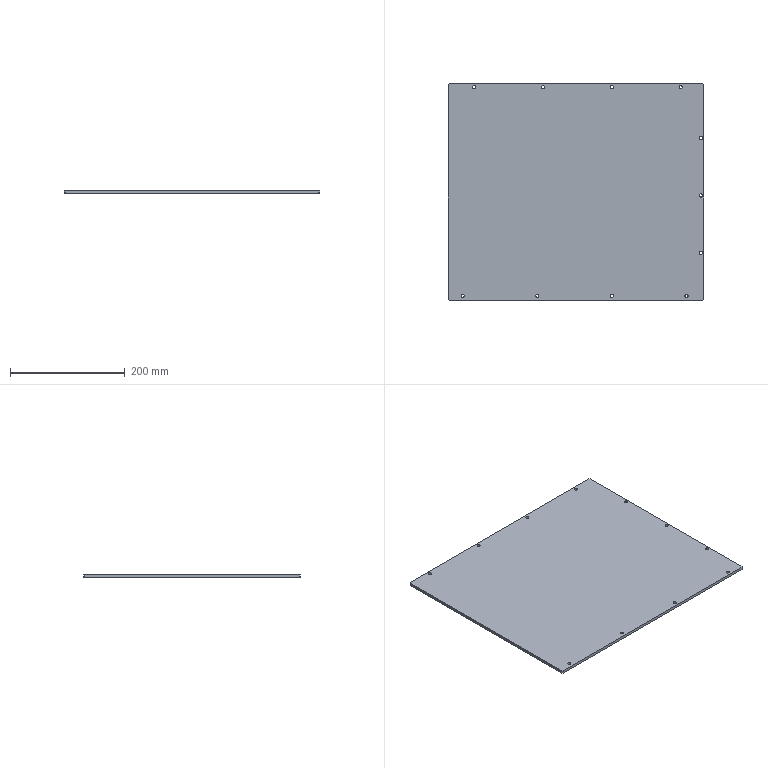Part | SolidWorks | features Extrusion 1, Fillet 1, HoleWzd 1 | 1 solid | 32 faces | box 445 x 377 x 5 mm | volume 837478 mm3 | cylinder 22 | plane 10 | commonest cylinder face diameters 5.5 x22
STEP:
#1=CARTESIAN_POINT('',(-180.25,182.5,0.));
#2=VERTEX_POINT('',#1);
#3=CARTESIAN_POINT('',(-174.75,182.5,0.));
#4=VERTEX_POINT('',#3);
#5=CARTESIAN_POINT('',(-177.5,182.5,0.));
#6=DIRECTION('',(0.,0.,1.));
#7=DIRECTION('',(1.,0.,0.));
#8=AXIS2_PLACEMENT_3D('',#5,#6,#7);
#9=CIRCLE('',#8,2.75);
#10=EDGE_CURVE('',#2,#4,#9,.T.);
#11=ORIENTED_EDGE('',*,*,#10,.F.);
#12=CARTESIAN_POINT('',(-180.25,182.5,5.));
#13=VERTEX_POINT('',#12);
#14=CARTESIAN_POINT('',(-180.25,182.5,5.));
#15=DIRECTION('',(0.,0.,1.));
#16=VECTOR('',#15,1000.);
#17=LINE('',#14,#16);
#18=EDGE_CURVE('',#2,#13,#17,.T.);
#19=ORIENTED_EDGE('',*,*,#18,.T.);
#20=CARTESIAN_POINT('',(-174.75,182.5,5.));
#21=VERTEX_POINT('',#20);
#22=CARTESIAN_POINT('',(-177.5,182.5,5.));
#23=DIRECTION('',(0.,0.,1.));
#24=DIRECTION('',(1.,0.,0.));
#25=AXIS2_PLACEMENT_3D('',#22,#23,#24);
#26=CIRCLE('',#25,2.75);
#27=EDGE_CURVE('',#13,#21,#26,.T.);
#28=ORIENTED_EDGE('',*,*,#27,.T.);
#29=CARTESIAN_POINT('',(-174.75,182.5,5.));
#30=DIRECTION('',(0.,0.,1.));
#31=VECTOR('',#30,1000.);
#32=LINE('',#29,#31);
#33=EDGE_CURVE('',#4,#21,#32,.T.);
#34=ORIENTED_EDGE('',*,*,#33,.F.);
#35=EDGE_LOOP('',(#11,#19,#28,#34));
#36=FACE_OUTER_BOUND('',#35,.T.);
#37=CARTESIAN_POINT('',(-177.5,182.5,5.));
#38=DIRECTION('',(0.,0.,1.));
#39=DIRECTION('',(1.,0.,0.));
#40=AXIS2_PLACEMENT_3D('',#37,#38,#39);
#41=CYLINDRICAL_SURFACE('',#40,2.75);
#42=ADVANCED_FACE('',(#36),#41,.F.);
#43=CARTESIAN_POINT('',(-60.25,182.5,0.));
#44=VERTEX_POINT('',#43);
#45=CARTESIAN_POINT('',(-54.75,182.5,0.));
#46=VERTEX_POINT('',#45);
#47=CARTESIAN_POINT('',(-57.5,182.5,0.));
#48=DIRECTION('',(0.,0.,1.));
#49=DIRECTION('',(1.,0.,0.));
#50=AXIS2_PLACEMENT_3D('',#47,#48,#49);
#51=CIRCLE('',#50,2.75);
#52=EDGE_CURVE('',#44,#46,#51,.T.);
#53=ORIENTED_EDGE('',*,*,#52,.F.);
#54=CARTESIAN_POINT('',(-60.25,182.5,5.));
#55=VERTEX_POINT('',#54);
#56=CARTESIAN_POINT('',(-60.25,182.5,5.));
#57=DIRECTION('',(0.,0.,1.));
#58=VECTOR('',#57,1000.);
#59=LINE('',#56,#58);
#60=EDGE_CURVE('',#44,#55,#59,.T.);
#61=ORIENTED_EDGE('',*,*,#60,.T.);
#62=CARTESIAN_POINT('',(-54.75,182.5,5.));
#63=VERTEX_POINT('',#62);
#64=CARTESIAN_POINT('',(-57.5,182.5,5.));
#65=DIRECTION('',(0.,0.,1.));
#66=DIRECTION('',(1.,0.,0.));
#67=AXIS2_PLACEMENT_3D('',#64,#65,#66);
#68=CIRCLE('',#67,2.75);
#69=EDGE_CURVE('',#55,#63,#68,.T.);
#70=ORIENTED_EDGE('',*,*,#69,.T.);
#71=CARTESIAN_POINT('',(-54.75,182.5,5.));
#72=DIRECTION('',(0.,0.,1.));
#73=VECTOR('',#72,1000.);
#74=LINE('',#71,#73);
#75=EDGE_CURVE('',#46,#63,#74,.T.);
#76=ORIENTED_EDGE('',*,*,#75,.F.);
#77=EDGE_LOOP('',(#53,#61,#70,#76));
#78=FACE_OUTER_BOUND('',#77,.T.);
#79=CARTESIAN_POINT('',(-57.5,182.5,5.));
#80=DIRECTION('',(0.,0.,1.));
#81=DIRECTION('',(1.,0.,0.));
#82=AXIS2_PLACEMENT_3D('',#79,#80,#81);
#83=CYLINDRICAL_SURFACE('',#82,2.75);
#84=ADVANCED_FACE('',(#78),#83,.F.);
#85=CARTESIAN_POINT('',(59.75,182.5,0.));
#86=VERTEX_POINT('',#85);
#87=CARTESIAN_POINT('',(65.25,182.5,0.));
#88=VERTEX_POINT('',#87);
#89=CARTESIAN_POINT('',(62.5,182.5,0.));
#90=DIRECTION('',(0.,0.,1.));
#91=DIRECTION('',(1.,0.,0.));
#92=AXIS2_PLACEMENT_3D('',#89,#90,#91);
#93=CIRCLE('',#92,2.75);
#94=EDGE_CURVE('',#86,#88,#93,.T.);
#95=ORIENTED_EDGE('',*,*,#94,.F.);
#96=CARTESIAN_POINT('',(59.75,182.5,5.));
#97=VERTEX_POINT('',#96);
#98=CARTESIAN_POINT('',(59.75,182.5,5.));
#99=DIRECTION('',(0.,0.,1.));
#100=VECTOR('',#99,1000.);
#101=LINE('',#98,#100);
#102=EDGE_CURVE('',#86,#97,#101,.T.);
#103=ORIENTED_EDGE('',*,*,#102,.T.);
#104=CARTESIAN_POINT('',(65.25,182.5,5.));
#105=VERTEX_POINT('',#104);
#106=CARTESIAN_POINT('',(62.5,182.5,5.));
#107=DIRECTION('',(0.,0.,1.));
#108=DIRECTION('',(1.,0.,0.));
#109=AXIS2_PLACEMENT_3D('',#106,#107,#108);
#110=CIRCLE('',#109,2.75);
#111=EDGE_CURVE('',#97,#105,#110,.T.);
#112=ORIENTED_EDGE('',*,*,#111,.T.);
#113=CARTESIAN_POINT('',(65.25,182.5,5.));
#114=DIRECTION('',(0.,0.,1.));
#115=VECTOR('',#114,1000.);
#116=LINE('',#113,#115);
#117=EDGE_CURVE('',#88,#105,#116,.T.);
#118=ORIENTED_EDGE('',*,*,#117,.F.);
#119=EDGE_LOOP('',(#95,#103,#112,#118));
#120=FACE_OUTER_BOUND('',#119,.T.);
#121=CARTESIAN_POINT('',(62.5,182.5,5.));
#122=DIRECTION('',(0.,0.,1.));
#123=DIRECTION('',(1.,0.,0.));
#124=AXIS2_PLACEMENT_3D('',#121,#122,#123);
#125=CYLINDRICAL_SURFACE('',#124,2.75);
#126=ADVANCED_FACE('',(#120),#125,.F.);
#127=CARTESIAN_POINT('',(179.75,182.5,0.));
#128=VERTEX_POINT('',#127);
#129=CARTESIAN_POINT('',(185.25,182.5,0.));
#130=VERTEX_POINT('',#129);
#131=CARTESIAN_POINT('',(182.5,182.5,0.));
#132=DIRECTION('',(0.,0.,1.));
#133=DIRECTION('',(1.,0.,0.));
#134=AXIS2_PLACEMENT_3D('',#131,#132,#133);
#135=CIRCLE('',#134,2.75);
#136=EDGE_CURVE('',#128,#130,#135,.T.);
#137=ORIENTED_EDGE('',*,*,#136,.F.);
#138=CARTESIAN_POINT('',(179.75,182.5,5.));
#139=VERTEX_POINT('',#138);
#140=CARTESIAN_POINT('',(179.75,182.5,5.));
#141=DIRECTION('',(0.,0.,1.));
#142=VECTOR('',#141,1000.);
#143=LINE('',#140,#142);
#144=EDGE_CURVE('',#128,#139,#143,.T.);
#145=ORIENTED_EDGE('',*,*,#144,.T.);
#146=CARTESIAN_POINT('',(185.25,182.5,5.));
#147=VERTEX_POINT('',#146);
#148=CARTESIAN_POINT('',(182.5,182.5,5.));
#149=DIRECTION('',(0.,0.,1.));
#150=DIRECTION('',(1.,0.,0.));
#151=AXIS2_PLACEMENT_3D('',#148,#149,#150);
#152=CIRCLE('',#151,2.75);
#153=EDGE_CURVE('',#139,#147,#152,.T.);
#154=ORIENTED_EDGE('',*,*,#153,.T.);
#155=CARTESIAN_POINT('',(185.25,182.5,5.));
#156=DIRECTION('',(0.,0.,1.));
#157=VECTOR('',#156,1000.);
#158=LINE('',#155,#157);
#159=EDGE_CURVE('',#130,#147,#158,.T.);
#160=ORIENTED_EDGE('',*,*,#159,.F.);
#161=EDGE_LOOP('',(#137,#145,#154,#160));
#162=FACE_OUTER_BOUND('',#161,.T.);
#163=CARTESIAN_POINT('',(182.5,182.5,5.));
#164=DIRECTION('',(0.,0.,1.));
#165=DIRECTION('',(1.,0.,0.));
#166=AXIS2_PLACEMENT_3D('',#163,#164,#165);
#167=CYLINDRICAL_SURFACE('',#166,2.75);
#168=ADVANCED_FACE('',(#162),#167,.F.);
#169=CARTESIAN_POINT('',(-200.25,-181.,0.));
#170=VERTEX_POINT('',#169);
#171=CARTESIAN_POINT('',(-194.75,-181.,0.));
#172=VERTEX_POINT('',#171);
#173=CARTESIAN_POINT('',(-197.5,-181.,0.));
#174=DIRECTION('',(0.,0.,1.));
#175=DIRECTION('',(1.,0.,0.));
#176=AXIS2_PLACEMENT_3D('',#173,#174,#175);
#177=CIRCLE('',#176,2.75);
#178=EDGE_CURVE('',#170,#172,#177,.T.);
#179=ORIENTED_EDGE('',*,*,#178,.F.);
#180=CARTESIAN_POINT('',(-200.25,-181.,5.));
#181=VERTEX_POINT('',#180);
#182=CARTESIAN_POINT('',(-200.25,-181.,5.));
#183=DIRECTION('',(0.,0.,1.));
#184=VECTOR('',#183,1000.);
#185=LINE('',#182,#184);
#186=EDGE_CURVE('',#170,#181,#185,.T.);
#187=ORIENTED_EDGE('',*,*,#186,.T.);
#188=CARTESIAN_POINT('',(-194.75,-181.,5.));
#189=VERTEX_POINT('',#188);
#190=CARTESIAN_POINT('',(-197.5,-181.,5.));
#191=DIRECTION('',(0.,0.,1.));
#192=DIRECTION('',(1.,0.,0.));
#193=AXIS2_PLACEMENT_3D('',#190,#191,#192);
#194=CIRCLE('',#193,2.75);
#195=EDGE_CURVE('',#181,#189,#194,.T.);
#196=ORIENTED_EDGE('',*,*,#195,.T.);
#197=CARTESIAN_POINT('',(-194.75,-181.,5.));
#198=DIRECTION('',(0.,0.,1.));
#199=VECTOR('',#198,1000.);
#200=LINE('',#197,#199);
#201=EDGE_CURVE('',#172,#189,#200,.T.);
#202=ORIENTED_EDGE('',*,*,#201,.F.);
#203=EDGE_LOOP('',(#179,#187,#196,#202));
#204=FACE_OUTER_BOUND('',#203,.T.);
#205=CARTESIAN_POINT('',(-197.5,-181.,5.));
#206=DIRECTION('',(0.,0.,1.));
#207=DIRECTION('',(1.,0.,0.));
#208=AXIS2_PLACEMENT_3D('',#205,#206,#207);
#209=CYLINDRICAL_SURFACE('',#208,2.75);
#210=ADVANCED_FACE('',(#204),#209,.F.);
#211=CARTESIAN_POINT('',(-70.25,-181.,0.));
#212=VERTEX_POINT('',#211);
#213=CARTESIAN_POINT('',(-64.75,-181.,0.));
#214=VERTEX_POINT('',#213);
#215=CARTESIAN_POINT('',(-67.5,-181.,0.));
#216=DIRECTION('',(0.,0.,1.));
#217=DIRECTION('',(1.,0.,0.));
#218=AXIS2_PLACEMENT_3D('',#215,#216,#217);
#219=CIRCLE('',#218,2.75);
#220=EDGE_CURVE('',#212,#214,#219,.T.);
#221=ORIENTED_EDGE('',*,*,#220,.F.);
#222=CARTESIAN_POINT('',(-70.25,-181.,5.));
#223=VERTEX_POINT('',#222);
#224=CARTESIAN_POINT('',(-70.25,-181.,5.));
#225=DIRECTION('',(0.,0.,1.));
#226=VECTOR('',#225,1000.);
#227=LINE('',#224,#226);
#228=EDGE_CURVE('',#212,#223,#227,.T.);
#229=ORIENTED_EDGE('',*,*,#228,.T.);
#230=CARTESIAN_POINT('',(-64.75,-181.,5.));
#231=VERTEX_POINT('',#230);
#232=CARTESIAN_POINT('',(-67.5,-181.,5.));
#233=DIRECTION('',(0.,0.,1.));
#234=DIRECTION('',(1.,0.,0.));
#235=AXIS2_PLACEMENT_3D('',#232,#233,#234);
#236=CIRCLE('',#235,2.75);
#237=EDGE_CURVE('',#223,#231,#236,.T.);
#238=ORIENTED_EDGE('',*,*,#237,.T.);
#239=CARTESIAN_POINT('',(-64.75,-181.,5.));
#240=DIRECTION('',(0.,0.,1.));
#241=VECTOR('',#240,1000.);
#242=LINE('',#239,#241);
#243=EDGE_CURVE('',#214,#231,#242,.T.);
#244=ORIENTED_EDGE('',*,*,#243,.F.);
#245=EDGE_LOOP('',(#221,#229,#238,#244));
#246=FACE_OUTER_BOUND('',#245,.T.);
#247=CARTESIAN_POINT('',(-67.5,-181.,5.));
#248=DIRECTION('',(0.,0.,1.));
#249=DIRECTION('',(1.,0.,0.));
#250=AXIS2_PLACEMENT_3D('',#247,#248,#249);
#251=CYLINDRICAL_SURFACE('',#250,2.75);
#252=ADVANCED_FACE('',(#246),#251,.F.);
#253=CARTESIAN_POINT('',(59.75,-181.,0.));
#254=VERTEX_POINT('',#253);
#255=CARTESIAN_POINT('',(65.25,-181.,0.));
#256=VERTEX_POINT('',#255);
#257=CARTESIAN_POINT('',(62.5,-181.,0.));
#258=DIRECTION('',(0.,0.,1.));
#259=DIRECTION('',(1.,0.,0.));
#260=AXIS2_PLACEMENT_3D('',#257,#258,#259);
#261=CIRCLE('',#260,2.75);
#262=EDGE_CURVE('',#254,#256,#261,.T.);
#263=ORIENTED_EDGE('',*,*,#262,.F.);
#264=CARTESIAN_POINT('',(59.75,-181.,5.));
#265=VERTEX_POINT('',#264);
#266=CARTESIAN_POINT('',(59.75,-181.,5.));
#267=DIRECTION('',(0.,0.,1.));
#268=VECTOR('',#267,1000.);
#269=LINE('',#266,#268);
#270=EDGE_CURVE('',#254,#265,#269,.T.);
#271=ORIENTED_EDGE('',*,*,#270,.T.);
#272=CARTESIAN_POINT('',(65.25,-181.,5.));
#273=VERTEX_POINT('',#272);
#274=CARTESIAN_POINT('',(62.5,-181.,5.));
#275=DIRECTION('',(0.,0.,1.));
#276=DIRECTION('',(1.,0.,0.));
#277=AXIS2_PLACEMENT_3D('',#274,#275,#276);
#278=CIRCLE('',#277,2.75);
#279=EDGE_CURVE('',#265,#273,#278,.T.);
#280=ORIENTED_EDGE('',*,*,#279,.T.);
#281=CARTESIAN_POINT('',(65.25,-181.,5.));
#282=DIRECTION('',(0.,0.,1.));
#283=VECTOR('',#282,1000.);
#284=LINE('',#281,#283);
#285=EDGE_CURVE('',#256,#273,#284,.T.);
#286=ORIENTED_EDGE('',*,*,#285,.F.);
#287=EDGE_LOOP('',(#263,#271,#280,#286));
#288=FACE_OUTER_BOUND('',#287,.T.);
#289=CARTESIAN_POINT('',(62.5,-181.,5.));
#290=DIRECTION('',(0.,0.,1.));
#291=DIRECTION('',(1.,0.,0.));
#292=AXIS2_PLACEMENT_3D('',#289,#290,#291);
#293=CYLINDRICAL_SURFACE('',#292,2.75);
#294=ADVANCED_FACE('',(#288),#293,.F.);
#295=CARTESIAN_POINT('',(189.75,-181.,0.));
#296=VERTEX_POINT('',#295);
#297=CARTESIAN_POINT('',(195.25,-181.,0.));
#298=VERTEX_POINT('',#297);
#299=CARTESIAN_POINT('',(192.5,-181.,0.));
#300=DIRECTION('',(0.,0.,1.));
#301=DIRECTION('',(1.,0.,0.));
#302=AXIS2_PLACEMENT_3D('',#299,#300,#301);
#303=CIRCLE('',#302,2.75);
#304=EDGE_CURVE('',#296,#298,#303,.T.);
#305=ORIENTED_EDGE('',*,*,#304,.F.);
#306=CARTESIAN_POINT('',(189.75,-181.,5.));
#307=VERTEX_POINT('',#306);
#308=CARTESIAN_POINT('',(189.75,-181.,5.));
#309=DIRECTION('',(0.,0.,1.));
#310=VECTOR('',#309,1000.);
#311=LINE('',#308,#310);
#312=EDGE_CURVE('',#296,#307,#311,.T.);
#313=ORIENTED_EDGE('',*,*,#312,.T.);
#314=CARTESIAN_POINT('',(195.25,-181.,5.));
#315=VERTEX_POINT('',#314);
#316=CARTESIAN_POINT('',(192.5,-181.,5.));
#317=DIRECTION('',(0.,0.,1.));
#318=DIRECTION('',(1.,0.,0.));
#319=AXIS2_PLACEMENT_3D('',#316,#317,#318);
#320=CIRCLE('',#319,2.75);
#321=EDGE_CURVE('',#307,#315,#320,.T.);
#322=ORIENTED_EDGE('',*,*,#321,.T.);
#323=CARTESIAN_POINT('',(195.25,-181.,5.));
#324=DIRECTION('',(0.,0.,1.));
#325=VECTOR('',#324,1000.);
#326=LINE('',#323,#325);
#327=EDGE_CURVE('',#298,#315,#326,.T.);
#328=ORIENTED_EDGE('',*,*,#327,.F.);
#329=EDGE_LOOP('',(#305,#313,#322,#328));
#330=FACE_OUTER_BOUND('',#329,.T.);
#331=CARTESIAN_POINT('',(192.5,-181.,5.));
#332=DIRECTION('',(0.,0.,1.));
#333=DIRECTION('',(1.,0.,0.));
#334=AXIS2_PLACEMENT_3D('',#331,#332,#333);
#335=CYLINDRICAL_SURFACE('',#334,2.75);
#336=ADVANCED_FACE('',(#330),#335,.F.);
#337=CARTESIAN_POINT('',(214.75,-106.,0.));
#338=VERTEX_POINT('',#337);
#339=CARTESIAN_POINT('',(220.25,-106.,0.));
#340=VERTEX_POINT('',#339);
#341=CARTESIAN_POINT('',(217.5,-106.,0.));
#342=DIRECTION('',(0.,0.,1.));
#343=DIRECTION('',(1.,0.,0.));
#344=AXIS2_PLACEMENT_3D('',#341,#342,#343);
#345=CIRCLE('',#344,2.75);
#346=EDGE_CURVE('',#338,#340,#345,.T.);
#347=ORIENTED_EDGE('',*,*,#346,.F.);
#348=CARTESIAN_POINT('',(214.75,-106.,5.));
#349=VERTEX_POINT('',#348);
#350=CARTESIAN_POINT('',(214.75,-106.,5.));
#351=DIRECTION('',(0.,0.,1.));
#352=VECTOR('',#351,1000.);
#353=LINE('',#350,#352);
#354=EDGE_CURVE('',#338,#349,#353,.T.);
#355=ORIENTED_EDGE('',*,*,#354,.T.);
#356=CARTESIAN_POINT('',(220.25,-106.,5.));
#357=VERTEX_POINT('',#356);
#358=CARTESIAN_POINT('',(217.5,-106.,5.));
#359=DIRECTION('',(0.,0.,1.));
#360=DIRECTION('',(1.,0.,0.));
#361=AXIS2_PLACEMENT_3D('',#358,#359,#360);
#362=CIRCLE('',#361,2.75);
#363=EDGE_CURVE('',#349,#357,#362,.T.);
#364=ORIENTED_EDGE('',*,*,#363,.T.);
#365=CARTESIAN_POINT('',(220.25,-106.,5.));
#366=DIRECTION('',(0.,0.,1.));
#367=VECTOR('',#366,1000.);
#368=LINE('',#365,#367);
#369=EDGE_CURVE('',#340,#357,#368,.T.);
#370=ORIENTED_EDGE('',*,*,#369,.F.);
#371=EDGE_LOOP('',(#347,#355,#364,#370));
#372=FACE_OUTER_BOUND('',#371,.T.);
#373=CARTESIAN_POINT('',(217.5,-106.,5.));
#374=DIRECTION('',(0.,0.,1.));
#375=DIRECTION('',(1.,0.,0.));
#376=AXIS2_PLACEMENT_3D('',#373,#374,#375);
#377=CYLINDRICAL_SURFACE('',#376,2.75);
#378=ADVANCED_FACE('',(#372),#377,.F.);
#379=CARTESIAN_POINT('',(214.75,-6.,0.));
#380=VERTEX_POINT('',#379);
#381=CARTESIAN_POINT('',(220.25,-6.,0.));
#382=VERTEX_POINT('',#381);
#383=CARTESIAN_POINT('',(217.5,-6.,0.));
#384=DIRECTION('',(0.,0.,1.));
#385=DIRECTION('',(1.,0.,0.));
#386=AXIS2_PLACEMENT_3D('',#383,#384,#385);
#387=CIRCLE('',#386,2.75);
#388=EDGE_CURVE('',#380,#382,#387,.T.);
#389=ORIENTED_EDGE('',*,*,#388,.F.);
#390=CARTESIAN_POINT('',(214.75,-6.,5.));
#391=VERTEX_POINT('',#390);
#392=CARTESIAN_POINT('',(214.75,-6.,5.));
#393=DIRECTION('',(0.,0.,1.));
#394=VECTOR('',#393,1000.);
#395=LINE('',#392,#394);
#396=EDGE_CURVE('',#380,#391,#395,.T.);
#397=ORIENTED_EDGE('',*,*,#396,.T.);
#398=CARTESIAN_POINT('',(220.25,-6.,5.));
#399=VERTEX_POINT('',#398);
#400=CARTESIAN_POINT('',(217.5,-6.,5.));
#401=DIRECTION('',(0.,0.,1.));
#402=DIRECTION('',(1.,0.,0.));
#403=AXIS2_PLACEMENT_3D('',#400,#401,#402);
#404=CIRCLE('',#403,2.75);
#405=EDGE_CURVE('',#391,#399,#404,.T.);
#406=ORIENTED_EDGE('',*,*,#405,.T.);
#407=CARTESIAN_POINT('',(220.25,-6.,5.));
#408=DIRECTION('',(0.,0.,1.));
#409=VECTOR('',#408,1000.);
#410=LINE('',#407,#409);
#411=EDGE_CURVE('',#382,#399,#410,.T.);
#412=ORIENTED_EDGE('',*,*,#411,.F.);
#413=EDGE_LOOP('',(#389,#397,#406,#412));
#414=FACE_OUTER_BOUND('',#413,.T.);
#415=CARTESIAN_POINT('',(217.5,-6.,5.));
#416=DIRECTION('',(0.,0.,1.));
#417=DIRECTION('',(1.,0.,0.));
#418=AXIS2_PLACEMENT_3D('',#415,#416,#417);
#419=CYLINDRICAL_SURFACE('',#418,2.75);
#420=ADVANCED_FACE('',(#414),#419,.F.);
#421=CARTESIAN_POINT('',(214.75,94.,0.));
#422=VERTEX_POINT('',#421);
#423=CARTESIAN_POINT('',(220.25,94.,0.));
#424=VERTEX_POINT('',#423);
#425=CARTESIAN_POINT('',(217.5,94.,0.));
#426=DIRECTION('',(0.,0.,1.));
#427=DIRECTION('',(1.,0.,0.));
#428=AXIS2_PLACEMENT_3D('',#425,#426,#427);
#429=CIRCLE('',#428,2.75);
#430=EDGE_CURVE('',#422,#424,#429,.T.);
#431=ORIENTED_EDGE('',*,*,#430,.F.);
#432=CARTESIAN_POINT('',(214.75,94.,5.));
#433=VERTEX_POINT('',#432);
#434=CARTESIAN_POINT('',(214.75,94.,5.));
#435=DIRECTION('',(0.,0.,1.));
#436=VECTOR('',#435,1000.);
#437=LINE('',#434,#436);
#438=EDGE_CURVE('',#422,#433,#437,.T.);
#439=ORIENTED_EDGE('',*,*,#438,.T.);
#440=CARTESIAN_POINT('',(220.25,94.,5.));
#441=VERTEX_POINT('',#440);
#442=CARTESIAN_POINT('',(217.5,94.,5.));
#443=DIRECTION('',(0.,0.,1.));
#444=DIRECTION('',(1.,0.,0.));
#445=AXIS2_PLACEMENT_3D('',#442,#443,#444);
#446=CIRCLE('',#445,2.75);
#447=EDGE_CURVE('',#433,#441,#446,.T.);
#448=ORIENTED_EDGE('',*,*,#447,.T.);
#449=CARTESIAN_POINT('',(220.25,94.,5.));
#450=DIRECTION('',(0.,0.,1.));
#451=VECTOR('',#450,1000.);
#452=LINE('',#449,#451);
#453=EDGE_CURVE('',#424,#441,#452,.T.);
#454=ORIENTED_EDGE('',*,*,#453,.F.);
#455=EDGE_LOOP('',(#431,#439,#448,#454));
#456=FACE_OUTER_BOUND('',#455,.T.);
#457=CARTESIAN_POINT('',(217.5,94.,5.));
#458=DIRECTION('',(0.,0.,1.));
#459=DIRECTION('',(1.,0.,0.));
#460=AXIS2_PLACEMENT_3D('',#457,#458,#459);
#461=CYLINDRICAL_SURFACE('',#460,2.75);
#462=ADVANCED_FACE('',(#456),#461,.F.);
#463=CARTESIAN_POINT('',(222.5,-186.5,5.));
#464=VERTEX_POINT('',#463);
#465=CARTESIAN_POINT('',(222.5,186.5,5.));
#466=VERTEX_POINT('',#465);
#467=CARTESIAN_POINT('',(222.5,188.5,5.));
#468=DIRECTION('',(0.,1.,0.));
#469=VECTOR('',#468,1000.);
#470=LINE('',#467,#469);
#471=EDGE_CURVE('',#464,#466,#470,.T.);
#472=ORIENTED_EDGE('',*,*,#471,.F.);
#473=CARTESIAN_POINT('',(222.5,-186.5,0.));
#474=VERTEX_POINT('',#473);
#475=CARTESIAN_POINT('',(222.5,-186.5,5.));
#476=DIRECTION('',(0.,0.,-1.));
#477=VECTOR('',#476,1000.);
#478=LINE('',#475,#477);
#479=EDGE_CURVE('',#464,#474,#478,.T.);
#480=ORIENTED_EDGE('',*,*,#479,.T.);
#481=CARTESIAN_POINT('',(222.5,186.5,0.));
#482=VERTEX_POINT('',#481);
#483=CARTESIAN_POINT('',(222.5,188.5,0.));
#484=DIRECTION('',(0.,1.,0.));
#485=VECTOR('',#484,1000.);
#486=LINE('',#483,#485);
#487=EDGE_CURVE('',#474,#482,#486,.T.);
#488=ORIENTED_EDGE('',*,*,#487,.T.);
#489=CARTESIAN_POINT('',(222.5,186.5,5.));
#490=DIRECTION('',(0.,0.,1.));
#491=VECTOR('',#490,1000.);
#492=LINE('',#489,#491);
#493=EDGE_CURVE('',#482,#466,#492,.T.);
#494=ORIENTED_EDGE('',*,*,#493,.T.);
#495=EDGE_LOOP('',(#472,#480,#488,#494));
#496=FACE_OUTER_BOUND('',#495,.T.);
#497=CARTESIAN_POINT('',(222.5,188.5,5.));
#498=DIRECTION('',(-1.,0.,0.));
#499=DIRECTION('',(0.,-1.,0.));
#500=AXIS2_PLACEMENT_3D('',#497,#498,#499);
#501=PLANE('',#500);
#502=ADVANCED_FACE('',(#496),#501,.F.);
#503=CARTESIAN_POINT('',(220.5,188.5,0.));
#504=VERTEX_POINT('',#503);
#505=CARTESIAN_POINT('',(-220.5,188.5,0.));
#506=VERTEX_POINT('',#505);
#507=CARTESIAN_POINT('',(-222.5,188.5,0.));
#508=DIRECTION('',(-1.,0.,0.));
#509=VECTOR('',#508,1000.);
#510=LINE('',#507,#509);
#511=EDGE_CURVE('',#504,#506,#510,.T.);
#512=ORIENTED_EDGE('',*,*,#511,.T.);
#513=CARTESIAN_POINT('',(-220.5,188.5,5.));
#514=VERTEX_POINT('',#513);
#515=CARTESIAN_POINT('',(-220.5,188.5,5.));
#516=DIRECTION('',(0.,0.,1.));
#517=VECTOR('',#516,1000.);
#518=LINE('',#515,#517);
#519=EDGE_CURVE('',#506,#514,#518,.T.);
#520=ORIENTED_EDGE('',*,*,#519,.T.);
#521=CARTESIAN_POINT('',(220.5,188.5,5.));
#522=VERTEX_POINT('',#521);
#523=CARTESIAN_POINT('',(-222.5,188.5,5.));
#524=DIRECTION('',(-1.,0.,0.));
#525=VECTOR('',#524,1000.);
#526=LINE('',#523,#525);
#527=EDGE_CURVE('',#522,#514,#526,.T.);
#528=ORIENTED_EDGE('',*,*,#527,.F.);
#529=CARTESIAN_POINT('',(220.5,188.5,5.));
#530=DIRECTION('',(0.,0.,-1.));
#531=VECTOR('',#530,1000.);
#532=LINE('',#529,#531);
#533=EDGE_CURVE('',#522,#504,#532,.T.);
#534=ORIENTED_EDGE('',*,*,#533,.T.);
#535=EDGE_LOOP('',(#512,#520,#528,#534));
#536=FACE_OUTER_BOUND('',#535,.T.);
#537=CARTESIAN_POINT('',(-222.5,188.5,5.));
#538=DIRECTION('',(0.,-1.,0.));
#539=DIRECTION('',(0.,0.,-1.));
#540=AXIS2_PLACEMENT_3D('',#537,#538,#539);
#541=PLANE('',#540);
#542=ADVANCED_FACE('',(#536),#541,.F.);
#543=CARTESIAN_POINT('',(-222.5,186.5,0.));
#544=VERTEX_POINT('',#543);
#545=CARTESIAN_POINT('',(-222.5,-186.5,0.));
#546=VERTEX_POINT('',#545);
#547=CARTESIAN_POINT('',(-222.5,188.5,0.));
#548=DIRECTION('',(0.,-1.,0.));
#549=VECTOR('',#548,1000.);
#550=LINE('',#547,#549);
#551=EDGE_CURVE('',#544,#546,#550,.T.);
#552=ORIENTED_EDGE('',*,*,#551,.T.);
#553=CARTESIAN_POINT('',(-222.5,-186.5,5.));
#554=VERTEX_POINT('',#553);
#555=CARTESIAN_POINT('',(-222.5,-186.5,5.));
#556=DIRECTION('',(0.,0.,1.));
#557=VECTOR('',#556,1000.);
#558=LINE('',#555,#557);
#559=EDGE_CURVE('',#546,#554,#558,.T.);
#560=ORIENTED_EDGE('',*,*,#559,.T.);
#561=CARTESIAN_POINT('',(-222.5,186.5,5.));
#562=VERTEX_POINT('',#561);
#563=CARTESIAN_POINT('',(-222.5,188.5,5.));
#564=DIRECTION('',(0.,-1.,0.));
#565=VECTOR('',#564,1000.);
#566=LINE('',#563,#565);
#567=EDGE_CURVE('',#562,#554,#566,.T.);
#568=ORIENTED_EDGE('',*,*,#567,.F.);
#569=CARTESIAN_POINT('',(-222.5,186.5,5.));
#570=DIRECTION('',(0.,0.,-1.));
#571=VECTOR('',#570,1000.);
#572=LINE('',#569,#571);
#573=EDGE_CURVE('',#562,#544,#572,.T.);
#574=ORIENTED_EDGE('',*,*,#573,.T.);
#575=EDGE_LOOP('',(#552,#560,#568,#574));
#576=FACE_OUTER_BOUND('',#575,.T.);
#577=CARTESIAN_POINT('',(-222.5,188.5,5.));
#578=DIRECTION('',(1.,0.,0.));
#579=DIRECTION('',(0.,1.,0.));
#580=AXIS2_PLACEMENT_3D('',#577,#578,#579);
#581=PLANE('',#580);
#582=ADVANCED_FACE('',(#576),#581,.F.);
#583=CARTESIAN_POINT('',(-220.5,-188.5,0.));
#584=VERTEX_POINT('',#583);
#585=CARTESIAN_POINT('',(220.5,-188.5,0.));
#586=VERTEX_POINT('',#585);
#587=CARTESIAN_POINT('',(-222.5,-188.5,0.));
#588=DIRECTION('',(1.,0.,0.));
#589=VECTOR('',#588,1000.);
#590=LINE('',#587,#589);
#591=EDGE_CURVE('',#584,#586,#590,.T.);
#592=ORIENTED_EDGE('',*,*,#591,.T.);
#593=CARTESIAN_POINT('',(220.5,-188.5,5.));
#594=VERTEX_POINT('',#593);
#595=CARTESIAN_POINT('',(220.5,-188.5,5.));
#596=DIRECTION('',(0.,0.,1.));
#597=VECTOR('',#596,1000.);
#598=LINE('',#595,#597);
#599=EDGE_CURVE('',#586,#594,#598,.T.);
#600=ORIENTED_EDGE('',*,*,#599,.T.);
#601=CARTESIAN_POINT('',(-220.5,-188.5,5.));
#602=VERTEX_POINT('',#601);
#603=CARTESIAN_POINT('',(-222.5,-188.5,5.));
#604=DIRECTION('',(1.,0.,0.));
#605=VECTOR('',#604,1000.);
#606=LINE('',#603,#605);
#607=EDGE_CURVE('',#602,#594,#606,.T.);
#608=ORIENTED_EDGE('',*,*,#607,.F.);
#609=CARTESIAN_POINT('',(-220.5,-188.5,5.));
#610=DIRECTION('',(0.,0.,-1.));
#611=VECTOR('',#610,1000.);
#612=LINE('',#609,#611);
#613=EDGE_CURVE('',#602,#584,#612,.T.);
#614=ORIENTED_EDGE('',*,*,#613,.T.);
#615=EDGE_LOOP('',(#592,#600,#608,#614));
#616=FACE_OUTER_BOUND('',#615,.T.);
#617=CARTESIAN_POINT('',(-222.5,-188.5,5.));
#618=DIRECTION('',(0.,1.,0.));
#619=DIRECTION('',(0.,0.,1.));
#620=AXIS2_PLACEMENT_3D('',#617,#618,#619);
#621=PLANE('',#620);
#622=ADVANCED_FACE('',(#616),#621,.F.);
#623=CARTESIAN_POINT('',(-177.5,182.5,5.));
#624=DIRECTION('',(0.,0.,1.));
#625=DIRECTION('',(1.,0.,0.));
#626=AXIS2_PLACEMENT_3D('',#623,#624,#625);
#627=CIRCLE('',#626,2.75);
#628=EDGE_CURVE('',#21,#13,#627,.T.);
#629=ORIENTED_EDGE('',*,*,#628,.F.);
#630=ORIENTED_EDGE('',*,*,#27,.F.);
#631=EDGE_LOOP('',(#629,#630));
#632=FACE_BOUND('',#631,.T.);
#633=CARTESIAN_POINT('',(-57.5,182.5,5.));
#634=DIRECTION('',(0.,0.,1.));
#635=DIRECTION('',(1.,0.,0.));
#636=AXIS2_PLACEMENT_3D('',#633,#634,#635);
#637=CIRCLE('',#636,2.75);
#638=EDGE_CURVE('',#63,#55,#637,.T.);
#639=ORIENTED_EDGE('',*,*,#638,.F.);
#640=ORIENTED_EDGE('',*,*,#69,.F.);
#641=EDGE_LOOP('',(#639,#640));
#642=FACE_BOUND('',#641,.T.);
#643=CARTESIAN_POINT('',(62.5,182.5,5.));
#644=DIRECTION('',(0.,0.,1.));
#645=DIRECTION('',(1.,0.,0.));
#646=AXIS2_PLACEMENT_3D('',#643,#644,#645);
#647=CIRCLE('',#646,2.75);
#648=EDGE_CURVE('',#105,#97,#647,.T.);
#649=ORIENTED_EDGE('',*,*,#648,.F.);
#650=ORIENTED_EDGE('',*,*,#111,.F.);
#651=EDGE_LOOP('',(#649,#650));
#652=FACE_BOUND('',#651,.T.);
#653=CARTESIAN_POINT('',(182.5,182.5,5.));
#654=DIRECTION('',(0.,0.,1.));
#655=DIRECTION('',(1.,0.,0.));
#656=AXIS2_PLACEMENT_3D('',#653,#654,#655);
#657=CIRCLE('',#656,2.75);
#658=EDGE_CURVE('',#147,#139,#657,.T.);
#659=ORIENTED_EDGE('',*,*,#658,.F.);
#660=ORIENTED_EDGE('',*,*,#153,.F.);
#661=EDGE_LOOP('',(#659,#660));
#662=FACE_BOUND('',#661,.T.);
#663=CARTESIAN_POINT('',(-197.5,-181.,5.));
#664=DIRECTION('',(0.,0.,1.));
#665=DIRECTION('',(1.,0.,0.));
#666=AXIS2_PLACEMENT_3D('',#663,#664,#665);
#667=CIRCLE('',#666,2.75);
#668=EDGE_CURVE('',#189,#181,#667,.T.);
#669=ORIENTED_EDGE('',*,*,#668,.F.);
#670=ORIENTED_EDGE('',*,*,#195,.F.);
#671=EDGE_LOOP('',(#669,#670));
#672=FACE_BOUND('',#671,.T.);
#673=CARTESIAN_POINT('',(-67.5,-181.,5.));
#674=DIRECTION('',(0.,0.,1.));
#675=DIRECTION('',(1.,0.,0.));
#676=AXIS2_PLACEMENT_3D('',#673,#674,#675);
#677=CIRCLE('',#676,2.75);
#678=EDGE_CURVE('',#231,#223,#677,.T.);
#679=ORIENTED_EDGE('',*,*,#678,.F.);
#680=ORIENTED_EDGE('',*,*,#237,.F.);
#681=EDGE_LOOP('',(#679,#680));
#682=FACE_BOUND('',#681,.T.);
#683=CARTESIAN_POINT('',(62.5,-181.,5.));
#684=DIRECTION('',(0.,0.,1.));
#685=DIRECTION('',(1.,0.,0.));
#686=AXIS2_PLACEMENT_3D('',#683,#684,#685);
#687=CIRCLE('',#686,2.75);
#688=EDGE_CURVE('',#273,#265,#687,.T.);
#689=ORIENTED_EDGE('',*,*,#688,.F.);
#690=ORIENTED_EDGE('',*,*,#279,.F.);
#691=EDGE_LOOP('',(#689,#690));
#692=FACE_BOUND('',#691,.T.);
#693=CARTESIAN_POINT('',(192.5,-181.,5.));
#694=DIRECTION('',(0.,0.,1.));
#695=DIRECTION('',(1.,0.,0.));
#696=AXIS2_PLACEMENT_3D('',#693,#694,#695);
#697=CIRCLE('',#696,2.75);
#698=EDGE_CURVE('',#315,#307,#697,.T.);
#699=ORIENTED_EDGE('',*,*,#698,.F.);
#700=ORIENTED_EDGE('',*,*,#321,.F.);
#701=EDGE_LOOP('',(#699,#700));
#702=FACE_BOUND('',#701,.T.);
#703=CARTESIAN_POINT('',(217.5,-106.,5.));
#704=DIRECTION('',(0.,0.,1.));
#705=DIRECTION('',(1.,0.,0.));
#706=AXIS2_PLACEMENT_3D('',#703,#704,#705);
#707=CIRCLE('',#706,2.75);
#708=EDGE_CURVE('',#357,#349,#707,.T.);
#709=ORIENTED_EDGE('',*,*,#708,.F.);
#710=ORIENTED_EDGE('',*,*,#363,.F.);
#711=EDGE_LOOP('',(#709,#710));
#712=FACE_BOUND('',#711,.T.);
#713=CARTESIAN_POINT('',(217.5,-6.,5.));
#714=DIRECTION('',(0.,0.,1.));
#715=DIRECTION('',(1.,0.,0.));
#716=AXIS2_PLACEMENT_3D('',#713,#714,#715);
#717=CIRCLE('',#716,2.75);
#718=EDGE_CURVE('',#399,#391,#717,.T.);
#719=ORIENTED_EDGE('',*,*,#718,.F.);
#720=ORIENTED_EDGE('',*,*,#405,.F.);
#721=EDGE_LOOP('',(#719,#720));
#722=FACE_BOUND('',#721,.T.);
#723=CARTESIAN_POINT('',(217.5,94.,5.));
#724=DIRECTION('',(0.,0.,1.));
#725=DIRECTION('',(1.,0.,0.));
#726=AXIS2_PLACEMENT_3D('',#723,#724,#725);
#727=CIRCLE('',#726,2.75);
#728=EDGE_CURVE('',#441,#433,#727,.T.);
#729=ORIENTED_EDGE('',*,*,#728,.F.);
#730=ORIENTED_EDGE('',*,*,#447,.F.);
#731=EDGE_LOOP('',(#729,#730));
#732=FACE_BOUND('',#731,.T.);
#733=ORIENTED_EDGE('',*,*,#607,.T.);
#734=CARTESIAN_POINT('',(204.5,-204.5,5.));
#735=DIRECTION('',(0.7071,0.7071,0.));
#736=VECTOR('',#735,1000.);
#737=LINE('',#734,#736);
#738=EDGE_CURVE('',#594,#464,#737,.T.);
#739=ORIENTED_EDGE('',*,*,#738,.T.);
#740=ORIENTED_EDGE('',*,*,#471,.T.);
#741=CARTESIAN_POINT('',(204.5,204.5,5.));
#742=DIRECTION('',(-0.7071,0.7071,0.));
#743=VECTOR('',#742,1000.);
#744=LINE('',#741,#743);
#745=EDGE_CURVE('',#466,#522,#744,.T.);
#746=ORIENTED_EDGE('',*,*,#745,.T.);
#747=ORIENTED_EDGE('',*,*,#527,.T.);
#748=CARTESIAN_POINT('',(-204.5,204.5,5.));
#749=DIRECTION('',(-0.7071,-0.7071,0.));
#750=VECTOR('',#749,1000.);
#751=LINE('',#748,#750);
#752=EDGE_CURVE('',#514,#562,#751,.T.);
#753=ORIENTED_EDGE('',*,*,#752,.T.);
#754=ORIENTED_EDGE('',*,*,#567,.T.);
#755=CARTESIAN_POINT('',(-204.5,-204.5,5.));
#756=DIRECTION('',(0.7071,-0.7071,0.));
#757=VECTOR('',#756,1000.);
#758=LINE('',#755,#757);
#759=EDGE_CURVE('',#554,#602,#758,.T.);
#760=ORIENTED_EDGE('',*,*,#759,.T.);
#761=EDGE_LOOP('',(#733,#739,#740,#746,#747,#753,#754,#760));
#762=FACE_OUTER_BOUND('',#761,.T.);
#763=CARTESIAN_POINT('',(0.,0.,5.));
#764=DIRECTION('',(0.,0.,1.));
#765=DIRECTION('',(1.,0.,0.));
#766=AXIS2_PLACEMENT_3D('',#763,#764,#765);
#767=PLANE('',#766);
#768=ADVANCED_FACE('',(#632,#642,#652,#662,#672,#682,#692,#702,#712,#722,#732,#762),#767,.T.);
#769=CARTESIAN_POINT('',(-177.5,182.5,0.));
#770=DIRECTION('',(0.,0.,1.));
#771=DIRECTION('',(1.,0.,0.));
#772=AXIS2_PLACEMENT_3D('',#769,#770,#771);
#773=CIRCLE('',#772,2.75);
#774=EDGE_CURVE('',#4,#2,#773,.T.);
#775=ORIENTED_EDGE('',*,*,#774,.T.);
#776=ORIENTED_EDGE('',*,*,#10,.T.);
#777=EDGE_LOOP('',(#775,#776));
#778=FACE_BOUND('',#777,.T.);
#779=CARTESIAN_POINT('',(-57.5,182.5,0.));
#780=DIRECTION('',(0.,0.,1.));
#781=DIRECTION('',(1.,0.,0.));
#782=AXIS2_PLACEMENT_3D('',#779,#780,#781);
#783=CIRCLE('',#782,2.75);
#784=EDGE_CURVE('',#46,#44,#783,.T.);
#785=ORIENTED_EDGE('',*,*,#784,.T.);
#786=ORIENTED_EDGE('',*,*,#52,.T.);
#787=EDGE_LOOP('',(#785,#786));
#788=FACE_BOUND('',#787,.T.);
#789=CARTESIAN_POINT('',(62.5,182.5,0.));
#790=DIRECTION('',(0.,0.,1.));
#791=DIRECTION('',(1.,0.,0.));
#792=AXIS2_PLACEMENT_3D('',#789,#790,#791);
#793=CIRCLE('',#792,2.75);
#794=EDGE_CURVE('',#88,#86,#793,.T.);
#795=ORIENTED_EDGE('',*,*,#794,.T.);
#796=ORIENTED_EDGE('',*,*,#94,.T.);
#797=EDGE_LOOP('',(#795,#796));
#798=FACE_BOUND('',#797,.T.);
#799=CARTESIAN_POINT('',(182.5,182.5,0.));
#800=DIRECTION('',(0.,0.,1.));
#801=DIRECTION('',(1.,0.,0.));
#802=AXIS2_PLACEMENT_3D('',#799,#800,#801);
#803=CIRCLE('',#802,2.75);
#804=EDGE_CURVE('',#130,#128,#803,.T.);
#805=ORIENTED_EDGE('',*,*,#804,.T.);
#806=ORIENTED_EDGE('',*,*,#136,.T.);
#807=EDGE_LOOP('',(#805,#806));
#808=FACE_BOUND('',#807,.T.);
#809=CARTESIAN_POINT('',(-197.5,-181.,0.));
#810=DIRECTION('',(0.,0.,1.));
#811=DIRECTION('',(1.,0.,0.));
#812=AXIS2_PLACEMENT_3D('',#809,#810,#811);
#813=CIRCLE('',#812,2.75);
#814=EDGE_CURVE('',#172,#170,#813,.T.);
#815=ORIENTED_EDGE('',*,*,#814,.T.);
#816=ORIENTED_EDGE('',*,*,#178,.T.);
#817=EDGE_LOOP('',(#815,#816));
#818=FACE_BOUND('',#817,.T.);
#819=CARTESIAN_POINT('',(-67.5,-181.,0.));
#820=DIRECTION('',(0.,0.,1.));
#821=DIRECTION('',(1.,0.,0.));
#822=AXIS2_PLACEMENT_3D('',#819,#820,#821);
#823=CIRCLE('',#822,2.75);
#824=EDGE_CURVE('',#214,#212,#823,.T.);
#825=ORIENTED_EDGE('',*,*,#824,.T.);
#826=ORIENTED_EDGE('',*,*,#220,.T.);
#827=EDGE_LOOP('',(#825,#826));
#828=FACE_BOUND('',#827,.T.);
#829=CARTESIAN_POINT('',(62.5,-181.,0.));
#830=DIRECTION('',(0.,0.,1.));
#831=DIRECTION('',(1.,0.,0.));
#832=AXIS2_PLACEMENT_3D('',#829,#830,#831);
#833=CIRCLE('',#832,2.75);
#834=EDGE_CURVE('',#256,#254,#833,.T.);
#835=ORIENTED_EDGE('',*,*,#834,.T.);
#836=ORIENTED_EDGE('',*,*,#262,.T.);
#837=EDGE_LOOP('',(#835,#836));
#838=FACE_BOUND('',#837,.T.);
#839=CARTESIAN_POINT('',(192.5,-181.,0.));
#840=DIRECTION('',(0.,0.,1.));
#841=DIRECTION('',(1.,0.,0.));
#842=AXIS2_PLACEMENT_3D('',#839,#840,#841);
#843=CIRCLE('',#842,2.75);
#844=EDGE_CURVE('',#298,#296,#843,.T.);
#845=ORIENTED_EDGE('',*,*,#844,.T.);
#846=ORIENTED_EDGE('',*,*,#304,.T.);
#847=EDGE_LOOP('',(#845,#846));
#848=FACE_BOUND('',#847,.T.);
#849=CARTESIAN_POINT('',(217.5,-106.,0.));
#850=DIRECTION('',(0.,0.,1.));
#851=DIRECTION('',(1.,0.,0.));
#852=AXIS2_PLACEMENT_3D('',#849,#850,#851);
#853=CIRCLE('',#852,2.75);
#854=EDGE_CURVE('',#340,#338,#853,.T.);
#855=ORIENTED_EDGE('',*,*,#854,.T.);
#856=ORIENTED_EDGE('',*,*,#346,.T.);
#857=EDGE_LOOP('',(#855,#856));
#858=FACE_BOUND('',#857,.T.);
#859=CARTESIAN_POINT('',(217.5,-6.,0.));
#860=DIRECTION('',(0.,0.,1.));
#861=DIRECTION('',(1.,0.,0.));
#862=AXIS2_PLACEMENT_3D('',#859,#860,#861);
#863=CIRCLE('',#862,2.75);
#864=EDGE_CURVE('',#382,#380,#863,.T.);
#865=ORIENTED_EDGE('',*,*,#864,.T.);
#866=ORIENTED_EDGE('',*,*,#388,.T.);
#867=EDGE_LOOP('',(#865,#866));
#868=FACE_BOUND('',#867,.T.);
#869=CARTESIAN_POINT('',(217.5,94.,0.));
#870=DIRECTION('',(0.,0.,1.));
#871=DIRECTION('',(1.,0.,0.));
#872=AXIS2_PLACEMENT_3D('',#869,#870,#871);
#873=CIRCLE('',#872,2.75);
#874=EDGE_CURVE('',#424,#422,#873,.T.);
#875=ORIENTED_EDGE('',*,*,#874,.T.);
#876=ORIENTED_EDGE('',*,*,#430,.T.);
#877=EDGE_LOOP('',(#875,#876));
#878=FACE_BOUND('',#877,.T.);
#879=ORIENTED_EDGE('',*,*,#487,.F.);
#880=CARTESIAN_POINT('',(222.5,-186.5,0.));
#881=DIRECTION('',(-0.7071,-0.7071,0.));
#882=VECTOR('',#881,1000.);
#883=LINE('',#880,#882);
#884=EDGE_CURVE('',#474,#586,#883,.T.);
#885=ORIENTED_EDGE('',*,*,#884,.T.);
#886=ORIENTED_EDGE('',*,*,#591,.F.);
#887=CARTESIAN_POINT('',(-220.5,-188.5,0.));
#888=DIRECTION('',(-0.7071,0.7071,0.));
#889=VECTOR('',#888,1000.);
#890=LINE('',#887,#889);
#891=EDGE_CURVE('',#584,#546,#890,.T.);
#892=ORIENTED_EDGE('',*,*,#891,.T.);
#893=ORIENTED_EDGE('',*,*,#551,.F.);
#894=CARTESIAN_POINT('',(-222.5,186.5,0.));
#895=DIRECTION('',(0.7071,0.7071,0.));
#896=VECTOR('',#895,1000.);
#897=LINE('',#894,#896);
#898=EDGE_CURVE('',#544,#506,#897,.T.);
#899=ORIENTED_EDGE('',*,*,#898,.T.);
#900=ORIENTED_EDGE('',*,*,#511,.F.);
#901=CARTESIAN_POINT('',(220.5,188.5,0.));
#902=DIRECTION('',(0.7071,-0.7071,0.));
#903=VECTOR('',#902,1000.);
#904=LINE('',#901,#903);
#905=EDGE_CURVE('',#504,#482,#904,.T.);
#906=ORIENTED_EDGE('',*,*,#905,.T.);
#907=EDGE_LOOP('',(#879,#885,#886,#892,#893,#899,#900,#906));
#908=FACE_OUTER_BOUND('',#907,.T.);
#909=CARTESIAN_POINT('',(0.,0.,0.));
#910=DIRECTION('',(0.,0.,1.));
#911=DIRECTION('',(1.,0.,0.));
#912=AXIS2_PLACEMENT_3D('',#909,#910,#911);
#913=PLANE('',#912);
#914=ADVANCED_FACE('',(#778,#788,#798,#808,#818,#828,#838,#848,#858,#868,#878,#908),#913,.F.);
#915=ORIENTED_EDGE('',*,*,#438,.F.);
#916=ORIENTED_EDGE('',*,*,#874,.F.);
#917=ORIENTED_EDGE('',*,*,#453,.T.);
#918=ORIENTED_EDGE('',*,*,#728,.T.);
#919=EDGE_LOOP('',(#915,#916,#917,#918));
#920=FACE_OUTER_BOUND('',#919,.T.);
#921=CARTESIAN_POINT('',(217.5,94.,5.));
#922=DIRECTION('',(0.,0.,1.));
#923=DIRECTION('',(1.,0.,0.));
#924=AXIS2_PLACEMENT_3D('',#921,#922,#923);
#925=CYLINDRICAL_SURFACE('',#924,2.75);
#926=ADVANCED_FACE('',(#920),#925,.F.);
#927=ORIENTED_EDGE('',*,*,#396,.F.);
#928=ORIENTED_EDGE('',*,*,#864,.F.);
#929=ORIENTED_EDGE('',*,*,#411,.T.);
#930=ORIENTED_EDGE('',*,*,#718,.T.);
#931=EDGE_LOOP('',(#927,#928,#929,#930));
#932=FACE_OUTER_BOUND('',#931,.T.);
#933=CARTESIAN_POINT('',(217.5,-6.,5.));
#934=DIRECTION('',(0.,0.,1.));
#935=DIRECTION('',(1.,0.,0.));
#936=AXIS2_PLACEMENT_3D('',#933,#934,#935);
#937=CYLINDRICAL_SURFACE('',#936,2.75);
#938=ADVANCED_FACE('',(#932),#937,.F.);
#939=ORIENTED_EDGE('',*,*,#354,.F.);
#940=ORIENTED_EDGE('',*,*,#854,.F.);
#941=ORIENTED_EDGE('',*,*,#369,.T.);
#942=ORIENTED_EDGE('',*,*,#708,.T.);
#943=EDGE_LOOP('',(#939,#940,#941,#942));
#944=FACE_OUTER_BOUND('',#943,.T.);
#945=CARTESIAN_POINT('',(217.5,-106.,5.));
#946=DIRECTION('',(0.,0.,1.));
#947=DIRECTION('',(1.,0.,0.));
#948=AXIS2_PLACEMENT_3D('',#945,#946,#947);
#949=CYLINDRICAL_SURFACE('',#948,2.75);
#950=ADVANCED_FACE('',(#944),#949,.F.);
#951=ORIENTED_EDGE('',*,*,#312,.F.);
#952=ORIENTED_EDGE('',*,*,#844,.F.);
#953=ORIENTED_EDGE('',*,*,#327,.T.);
#954=ORIENTED_EDGE('',*,*,#698,.T.);
#955=EDGE_LOOP('',(#951,#952,#953,#954));
#956=FACE_OUTER_BOUND('',#955,.T.);
#957=CARTESIAN_POINT('',(192.5,-181.,5.));
#958=DIRECTION('',(0.,0.,1.));
#959=DIRECTION('',(1.,0.,0.));
#960=AXIS2_PLACEMENT_3D('',#957,#958,#959);
#961=CYLINDRICAL_SURFACE('',#960,2.75);
#962=ADVANCED_FACE('',(#956),#961,.F.);
#963=ORIENTED_EDGE('',*,*,#270,.F.);
#964=ORIENTED_EDGE('',*,*,#834,.F.);
#965=ORIENTED_EDGE('',*,*,#285,.T.);
#966=ORIENTED_EDGE('',*,*,#688,.T.);
#967=EDGE_LOOP('',(#963,#964,#965,#966));
#968=FACE_OUTER_BOUND('',#967,.T.);
#969=CARTESIAN_POINT('',(62.5,-181.,5.));
#970=DIRECTION('',(0.,0.,1.));
#971=DIRECTION('',(1.,0.,0.));
#972=AXIS2_PLACEMENT_3D('',#969,#970,#971);
#973=CYLINDRICAL_SURFACE('',#972,2.75);
#974=ADVANCED_FACE('',(#968),#973,.F.);
#975=ORIENTED_EDGE('',*,*,#228,.F.);
#976=ORIENTED_EDGE('',*,*,#824,.F.);
#977=ORIENTED_EDGE('',*,*,#243,.T.);
#978=ORIENTED_EDGE('',*,*,#678,.T.);
#979=EDGE_LOOP('',(#975,#976,#977,#978));
#980=FACE_OUTER_BOUND('',#979,.T.);
#981=CARTESIAN_POINT('',(-67.5,-181.,5.));
#982=DIRECTION('',(0.,0.,1.));
#983=DIRECTION('',(1.,0.,0.));
#984=AXIS2_PLACEMENT_3D('',#981,#982,#983);
#985=CYLINDRICAL_SURFACE('',#984,2.75);
#986=ADVANCED_FACE('',(#980),#985,.F.);
#987=ORIENTED_EDGE('',*,*,#186,.F.);
#988=ORIENTED_EDGE('',*,*,#814,.F.);
#989=ORIENTED_EDGE('',*,*,#201,.T.);
#990=ORIENTED_EDGE('',*,*,#668,.T.);
#991=EDGE_LOOP('',(#987,#988,#989,#990));
#992=FACE_OUTER_BOUND('',#991,.T.);
#993=CARTESIAN_POINT('',(-197.5,-181.,5.));
#994=DIRECTION('',(0.,0.,1.));
#995=DIRECTION('',(1.,0.,0.));
#996=AXIS2_PLACEMENT_3D('',#993,#994,#995);
#997=CYLINDRICAL_SURFACE('',#996,2.75);
#998=ADVANCED_FACE('',(#992),#997,.F.);
#999=ORIENTED_EDGE('',*,*,#144,.F.);
#1000=ORIENTED_EDGE('',*,*,#804,.F.);
#1001=ORIENTED_EDGE('',*,*,#159,.T.);
#1002=ORIENTED_EDGE('',*,*,#658,.T.);
#1003=EDGE_LOOP('',(#999,#1000,#1001,#1002));
#1004=FACE_OUTER_BOUND('',#1003,.T.);
#1005=CARTESIAN_POINT('',(182.5,182.5,5.));
#1006=DIRECTION('',(0.,0.,1.));
#1007=DIRECTION('',(1.,0.,0.));
#1008=AXIS2_PLACEMENT_3D('',#1005,#1006,#1007);
#1009=CYLINDRICAL_SURFACE('',#1008,2.75);
#1010=ADVANCED_FACE('',(#1004),#1009,.F.);
#1011=ORIENTED_EDGE('',*,*,#102,.F.);
#1012=ORIENTED_EDGE('',*,*,#794,.F.);
#1013=ORIENTED_EDGE('',*,*,#117,.T.);
#1014=ORIENTED_EDGE('',*,*,#648,.T.);
#1015=EDGE_LOOP('',(#1011,#1012,#1013,#1014));
#1016=FACE_OUTER_BOUND('',#1015,.T.);
#1017=CARTESIAN_POINT('',(62.5,182.5,5.));
#1018=DIRECTION('',(0.,0.,1.));
#1019=DIRECTION('',(1.,0.,0.));
#1020=AXIS2_PLACEMENT_3D('',#1017,#1018,#1019);
#1021=CYLINDRICAL_SURFACE('',#1020,2.75);
#1022=ADVANCED_FACE('',(#1016),#1021,.F.);
#1023=ORIENTED_EDGE('',*,*,#60,.F.);
#1024=ORIENTED_EDGE('',*,*,#784,.F.);
#1025=ORIENTED_EDGE('',*,*,#75,.T.);
#1026=ORIENTED_EDGE('',*,*,#638,.T.);
#1027=EDGE_LOOP('',(#1023,#1024,#1025,#1026));
#1028=FACE_OUTER_BOUND('',#1027,.T.);
#1029=CARTESIAN_POINT('',(-57.5,182.5,5.));
#1030=DIRECTION('',(0.,0.,1.));
#1031=DIRECTION('',(1.,0.,0.));
#1032=AXIS2_PLACEMENT_3D('',#1029,#1030,#1031);
#1033=CYLINDRICAL_SURFACE('',#1032,2.75);
#1034=ADVANCED_FACE('',(#1028),#1033,.F.);
#1035=ORIENTED_EDGE('',*,*,#18,.F.);
#1036=ORIENTED_EDGE('',*,*,#774,.F.);
#1037=ORIENTED_EDGE('',*,*,#33,.T.);
#1038=ORIENTED_EDGE('',*,*,#628,.T.);
#1039=EDGE_LOOP('',(#1035,#1036,#1037,#1038));
#1040=FACE_OUTER_BOUND('',#1039,.T.);
#1041=CARTESIAN_POINT('',(-177.5,182.5,5.));
#1042=DIRECTION('',(0.,0.,1.));
#1043=DIRECTION('',(1.,0.,0.));
#1044=AXIS2_PLACEMENT_3D('',#1041,#1042,#1043);
#1045=CYLINDRICAL_SURFACE('',#1044,2.75);
#1046=ADVANCED_FACE('',(#1040),#1045,.F.);
#1047=ORIENTED_EDGE('',*,*,#738,.F.);
#1048=ORIENTED_EDGE('',*,*,#599,.F.);
#1049=ORIENTED_EDGE('',*,*,#884,.F.);
#1050=ORIENTED_EDGE('',*,*,#479,.F.);
#1051=EDGE_LOOP('',(#1047,#1048,#1049,#1050));
#1052=FACE_OUTER_BOUND('',#1051,.T.);
#1053=CARTESIAN_POINT('',(222.5,-186.5,5.));
#1054=DIRECTION('',(-0.7071,0.7071,0.));
#1055=DIRECTION('',(0.,0.,-1.));
#1056=AXIS2_PLACEMENT_3D('',#1053,#1054,#1055);
#1057=PLANE('',#1056);
#1058=ADVANCED_FACE('',(#1052),#1057,.F.);
#1059=ORIENTED_EDGE('',*,*,#759,.F.);
#1060=ORIENTED_EDGE('',*,*,#559,.F.);
#1061=ORIENTED_EDGE('',*,*,#891,.F.);
#1062=ORIENTED_EDGE('',*,*,#613,.F.);
#1063=EDGE_LOOP('',(#1059,#1060,#1061,#1062));
#1064=FACE_OUTER_BOUND('',#1063,.T.);
#1065=CARTESIAN_POINT('',(-220.5,-188.5,5.));
#1066=DIRECTION('',(0.7071,0.7071,0.));
#1067=DIRECTION('',(0.,0.,-1.));
#1068=AXIS2_PLACEMENT_3D('',#1065,#1066,#1067);
#1069=PLANE('',#1068);
#1070=ADVANCED_FACE('',(#1064),#1069,.F.);
#1071=ORIENTED_EDGE('',*,*,#752,.F.);
#1072=ORIENTED_EDGE('',*,*,#519,.F.);
#1073=ORIENTED_EDGE('',*,*,#898,.F.);
#1074=ORIENTED_EDGE('',*,*,#573,.F.);
#1075=EDGE_LOOP('',(#1071,#1072,#1073,#1074));
#1076=FACE_OUTER_BOUND('',#1075,.T.);
#1077=CARTESIAN_POINT('',(-222.5,186.5,5.));
#1078=DIRECTION('',(0.7071,-0.7071,0.));
#1079=DIRECTION('',(0.,0.,-1.));
#1080=AXIS2_PLACEMENT_3D('',#1077,#1078,#1079);
#1081=PLANE('',#1080);
#1082=ADVANCED_FACE('',(#1076),#1081,.F.);
#1083=ORIENTED_EDGE('',*,*,#745,.F.);
#1084=ORIENTED_EDGE('',*,*,#493,.F.);
#1085=ORIENTED_EDGE('',*,*,#905,.F.);
#1086=ORIENTED_EDGE('',*,*,#533,.F.);
#1087=EDGE_LOOP('',(#1083,#1084,#1085,#1086));
#1088=FACE_OUTER_BOUND('',#1087,.T.);
#1089=CARTESIAN_POINT('',(220.5,188.5,5.));
#1090=DIRECTION('',(-0.7071,-0.7071,0.));
#1091=DIRECTION('',(0.,0.,-1.));
#1092=AXIS2_PLACEMENT_3D('',#1089,#1090,#1091);
#1093=PLANE('',#1092);
#1094=ADVANCED_FACE('',(#1088),#1093,.F.);
#1095=CLOSED_SHELL('',(#42,#84,#126,#168,#210,#252,#294,#336,#378,#420,#462,#502,#542,#582,#622,#768,#914,#926,#938,#950,#962,#974,#986,#998,#1010,#1022,#1034,#1046,#1058,#1070,#1082,#1094));
#1096=MANIFOLD_SOLID_BREP('',#1095);
#1097=CARTESIAN_POINT('',(0.,0.,0.));
#1098=DIRECTION('',(0.,0.,1.));
#1099=DIRECTION('',(1.,0.,0.));
#1100=AXIS2_PLACEMENT_3D('',#1097,#1098,#1099);
#1101=(LENGTH_UNIT()NAMED_UNIT(*)SI_UNIT(.MILLI.,.METRE.));
#1102=UNCERTAINTY_MEASURE_WITH_UNIT(LENGTH_MEASURE(0.00001),#1101,'','');
#1103=(NAMED_UNIT(*)PLANE_ANGLE_UNIT()SI_UNIT($,.RADIAN.));
#1104=(NAMED_UNIT(*)SI_UNIT($,.STERADIAN.)SOLID_ANGLE_UNIT());
#1105=(GEOMETRIC_REPRESENTATION_CONTEXT(3)GLOBAL_UNCERTAINTY_ASSIGNED_CONTEXT((#1102))GLOBAL_UNIT_ASSIGNED_CONTEXT((#1101,#1103,#1104))REPRESENTATION_CONTEXT('',''));
#1106=ADVANCED_BREP_SHAPE_REPRESENTATION('',(#1096,#1100),#1105);